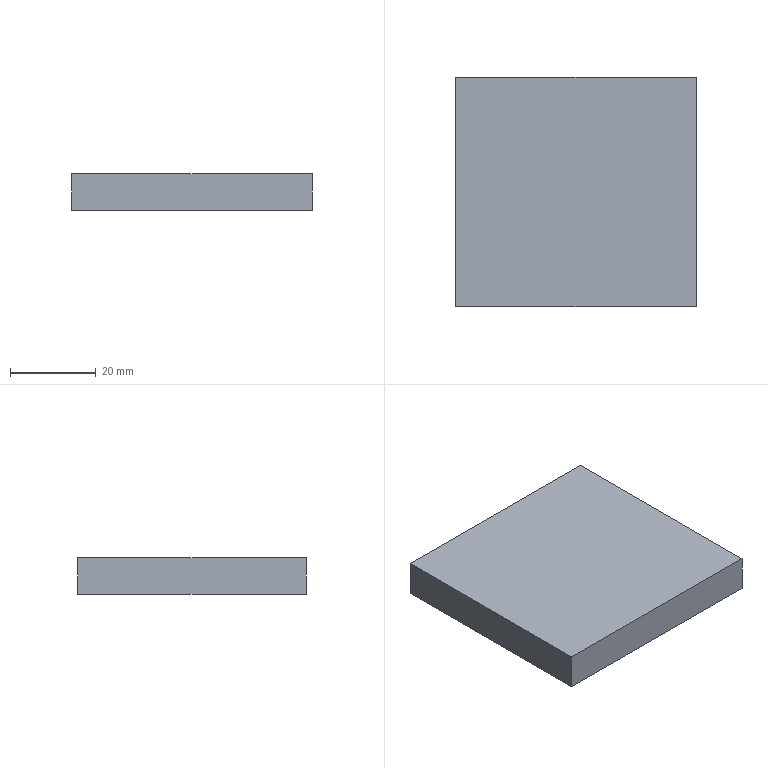NC program | NX | posted with a generic post | part box 56 x 53.3 x 8.5 mm
Lines 1846 to 3579 of 5023, first 1622 of 1730 lines:
(CAVITY_MILL_COPY , TOOL : D4)
N3678 T11 M6
N3680 G54
N3682 G17 G0 G90 X8.296 Y14.357 S9500 M3
N3684 G43 Z30. H11
N3686 Z-0.75
N3688 G94 G1 Z-1.75 F800.
N3690 X8.533 Y14.434
N3692 G3 X9.2 Y15.179 R1.
N3694 G2 X9.473 Y16.065 R5.05 F1200.
N3696 G3 X8.615 Y16.541 R18.65
N3698 X7.615 Y16.498 R1.
N3700 G1 X7.293 Y16.292
N3702 Z-0.75
N3704 X8.296 Y14.357 Z-1. F6000.
N3706 Z-2. F800.
N3708 X8.533 Y14.434
N3710 G3 X9.2 Y15.179 R1.
N3712 G2 X9.473 Y16.065 R5.05 F1200.
N3714 G3 X8.615 Y16.541 R18.65
N3716 X7.615 Y16.498 R1.
N3718 G1 X7.293 Y16.292
N3720 Z-1.
N3722 X8.296 Y14.357 Z-1.25 F6000.
N3724 Z-2.25 F800.
N3726 X8.533 Y14.434
N3728 G3 X9.2 Y15.179 R1.
N3730 G2 X9.473 Y16.065 R5.05 F1200.
N3732 G3 X8.615 Y16.541 R18.65
N3734 X7.615 Y16.498 R1.
N3736 G1 X7.293 Y16.292
N3738 Z-1.25
N3740 X8.296 Y14.357 Z-1.5 F6000.
N3742 Z-2.5 F800.
N3744 X8.533 Y14.434
N3746 G3 X9.2 Y15.179 R1.
N3748 G2 X9.473 Y16.065 R5.05 F1200.
N3750 G3 X8.615 Y16.541 R18.65
N3752 X7.615 Y16.498 R1.
N3754 G1 X7.293 Y16.292
N3756 Z-1.5
N3758 G0 Z30.
N3760 X15.388 Y16.801
N3762 Z-0.75
N3764 G1 Z-1.75 F800.
N3766 X15.171 Y16.699
N3768 G3 X14.599 Y15.878 R1.
N3770 G2 X14.098 Y14.165 R4.5 F1200.
N3772 G1 X14.072 Y14.116
N3774 X14.116 Y14.072
N3776 X14.165 Y14.098
N3778 G2 X15.878 Y14.599 R4.5
N3780 G3 X16.699 Y15.171 R1.
N3782 G1 X16.801 Y15.388
N3784 Z-0.75
N3786 X15.388 Y16.801 Z-1. F6000.
N3788 Z-2. F800.
N3790 X15.171 Y16.699
N3792 G3 X14.599 Y15.878 R1.
N3794 G2 X14.098 Y14.165 R4.5 F1200.
N3796 G1 X14.072 Y14.116
N3798 X14.116 Y14.072
N3800 X14.165 Y14.098
N3802 G2 X15.878 Y14.599 R4.5
N3804 G3 X16.699 Y15.171 R1.
N3806 G1 X16.801 Y15.388
N3808 Z-1.
N3810 X15.388 Y16.801 Z-1.25 F6000.
N3812 Z-2.25 F800.
N3814 X15.171 Y16.699
N3816 G3 X14.599 Y15.878 R1.
N3818 G2 X14.098 Y14.165 R4.5 F1200.
N3820 G1 X14.072 Y14.116
N3822 X14.116 Y14.072
N3824 X14.165 Y14.098
N3826 G2 X15.878 Y14.599 R4.5
N3828 G3 X16.699 Y15.171 R1.
N3830 G1 X16.801 Y15.388
N3832 Z-1.25
N3834 X15.388 Y16.801 Z-1.5 F6000.
N3836 Z-2.5 F800.
N3838 X15.171 Y16.699
N3840 G3 X14.599 Y15.878 R1.
N3842 G2 X14.098 Y14.165 R4.5 F1200.
N3844 G1 X14.072 Y14.116
N3846 X14.116 Y14.072
N3848 X14.165 Y14.098
N3850 G2 X15.878 Y14.599 R4.5
N3852 G3 X16.699 Y15.171 R1.
N3854 G1 X16.801 Y15.388
N3856 Z-1.5
N3858 X15.388 Y16.801 Z-1.8 F6000.
N3860 Z-2.8 F800.
N3862 X15.171 Y16.699
N3864 G3 X14.599 Y15.878 R1.
N3866 G2 X14.098 Y14.165 R4.5 F1200.
N3868 G1 X14.072 Y14.116
N3870 X14.116 Y14.072
N3872 X14.165 Y14.098
N3874 G2 X15.878 Y14.599 R4.5
N3876 G3 X16.699 Y15.171 R1.
N3878 G1 X16.801 Y15.388
N3880 Z-1.8
N3882 X15.388 Y16.801 Z-2.1 F6000.
N3884 Z-3.1 F800.
N3886 X15.171 Y16.699
N3888 G3 X14.599 Y15.878 R1.
N3890 G2 X14.098 Y14.165 R4.5 F1200.
N3892 G1 X14.072 Y14.116
N3894 X14.116 Y14.072
N3896 X14.165 Y14.098
N3898 G2 X15.878 Y14.599 R4.5
N3900 G3 X16.699 Y15.171 R1.
N3902 G1 X16.801 Y15.388
N3904 Z-2.1
N3906 X15.388 Y16.801 Z-2.3 F6000.
N3908 Z-3.3 F800.
N3910 X15.171 Y16.699
N3912 G3 X14.599 Y15.878 R1.
N3914 G2 X14.098 Y14.165 R4.5 F1200.
N3916 G1 X14.072 Y14.116
N3918 X14.116 Y14.072
N3920 X14.165 Y14.098
N3922 G2 X15.878 Y14.599 R4.5
N3924 G3 X16.699 Y15.171 R1.
N3926 G1 X16.801 Y15.388
N3928 Z-2.3
N3930 X15.388 Y16.801 Z-2.5 F6000.
N3932 Z-3.5 F800.
N3934 X15.171 Y16.699
N3936 G3 X14.599 Y15.878 R1.
N3938 G2 X14.098 Y14.165 R4.5 F1200.
N3940 G1 X14.072 Y14.116
N3942 X14.116 Y14.072
N3944 X14.165 Y14.098
N3946 G2 X15.878 Y14.599 R4.5
N3948 G3 X16.699 Y15.171 R1.
N3950 G1 X16.801 Y15.388
N3952 Z-2.5
N3954 G0 Z30.
N3956 X16.292 Y7.293
N3958 Z-0.75
N3960 G1 Z-1.75 F800.
N3962 X16.498 Y7.615
N3964 G3 X16.541 Y8.615 R1.
N3966 X16.065 Y9.473 R18.65 F1200.
N3968 G2 X15.179 Y9.2 R5.05
N3970 G3 X14.434 Y8.533 R1.
N3972 G1 X14.357 Y8.296
N3974 Z-0.75
N3976 X16.292 Y7.293 Z-1. F6000.
N3978 Z-2. F800.
N3980 X16.498 Y7.615
N3982 G3 X16.541 Y8.615 R1.
N3984 X16.065 Y9.473 R18.65 F1200.
N3986 G2 X15.179 Y9.2 R5.05
N3988 G3 X14.434 Y8.533 R1.
N3990 G1 X14.357 Y8.296
N3992 Z-1.
N3994 X16.292 Y7.293 Z-1.25 F6000.
N3996 Z-2.25 F800.
N3998 X16.498 Y7.615
N4000 G3 X16.541 Y8.615 R1.
N4002 X16.065 Y9.473 R18.65 F1200.
N4004 G2 X15.179 Y9.2 R5.05
N4006 G3 X14.434 Y8.533 R1.
N4008 G1 X14.357 Y8.296
N4010 Z-1.25
N4012 X16.292 Y7.293 Z-1.5 F6000.
N4014 Z-2.5 F800.
N4016 X16.498 Y7.615
N4018 G3 X16.541 Y8.615 R1.
N4020 X16.065 Y9.473 R18.65 F1200.
N4022 G2 X15.179 Y9.2 R5.05
N4024 G3 X14.434 Y8.533 R1.
N4026 G1 X14.357 Y8.296
N4028 Z-1.5
N4030 G0 Z30.
N4032 X21.661 Y11.34
N4034 Z-0.75
N4036 G1 Z-1.75 F800.
N4038 X21.478 Y11.076
N4040 G3 X21.394 Y10.08 R1.
N4042 G2 X21.665 Y9.484 R23.65 F1200.
N4044 X22.28 Y9.334 R2.5
N4046 G3 X23.267 Y9.49 R1.
N4048 G1 X23.409 Y9.605
N4050 Z-0.75
N4052 X21.661 Y11.34 Z-1. F6000.
N4054 Z-2. F800.
N4056 X21.478 Y11.076
N4058 G3 X21.394 Y10.08 R1.
N4060 G2 X21.665 Y9.484 R23.65 F1200.
N4062 X22.28 Y9.334 R2.5
N4064 G3 X23.267 Y9.49 R1.
N4066 G1 X23.409 Y9.605
N4068 Z-1.
N4070 X21.661 Y11.34 Z-1.25 F6000.
N4072 Z-2.25 F800.
N4074 X21.478 Y11.076
N4076 G3 X21.394 Y10.08 R1.
N4078 G2 X21.665 Y9.484 R23.65 F1200.
N4080 X22.28 Y9.334 R2.5
N4082 G3 X23.267 Y9.49 R1.
N4084 G1 X23.409 Y9.605
N4086 Z-1.25
N4088 X21.661 Y11.34 Z-1.5 F6000.
N4090 Z-2.5 F800.
N4092 X21.478 Y11.076
N4094 G3 X21.394 Y10.08 R1.
N4096 G2 X21.665 Y9.484 R23.65 F1200.
N4098 X22.28 Y9.334 R2.5
N4100 G3 X23.267 Y9.49 R1.
N4102 G1 X23.409 Y9.605
N4104 Z-1.5
N4106 X21.661 Y11.34 Z-1.8 F6000.
N4108 Z-2.8 F800.
N4110 X21.478 Y11.076
N4112 G3 X21.394 Y10.08 R1.
N4114 G2 X21.665 Y9.484 R23.65 F1200.
N4116 X22.28 Y9.334 R2.5
N4118 G3 X23.267 Y9.49 R1.
N4120 G1 X23.409 Y9.605
N4122 Z-1.8
N4124 X21.661 Y11.34 Z-2.1 F6000.
N4126 Z-3.1 F800.
N4128 X21.478 Y11.076
N4130 G3 X21.394 Y10.08 R1.
N4132 G2 X21.665 Y9.484 R23.65 F1200.
N4134 X22.28 Y9.334 R2.5
N4136 G3 X23.267 Y9.49 R1.
N4138 G1 X23.409 Y9.605
N4140 Z-2.1
N4142 X21.661 Y11.34 Z-2.3 F6000.
N4144 Z-3.3 F800.
N4146 X21.478 Y11.076
N4148 G3 X21.394 Y10.08 R1.
N4150 G2 X21.665 Y9.484 R23.65 F1200.
N4152 X22.28 Y9.334 R2.5
N4154 G3 X23.267 Y9.49 R1.
N4156 G1 X23.409 Y9.605
N4158 Z-2.3
N4160 X21.661 Y11.34 Z-2.5 F6000.
N4162 Z-3.5 F800.
N4164 X21.478 Y11.076
N4166 G3 X21.394 Y10.08 R1.
N4168 G2 X21.665 Y9.484 R23.65 F1200.
N4170 X22.28 Y9.334 R2.5
N4172 G3 X23.267 Y9.49 R1.
N4174 G1 X23.409 Y9.605
N4176 Z-2.5
N4178 G0 Z30.
N4180 X18.956 Y3.051
N4182 Z-0.75
N4184 G1 Z-1.75 F800.
N4186 X19.237 Y3.306
N4188 G3 X19.541 Y4.259 R1.
N4190 X19.4 Y4.863 R20. F1200.
N4192 G2 X18.864 Y5.142 R4.
N4194 G3 X17.865 Y5.176 R1.
N4196 G1 X17.662 Y5.068
N4198 Z-0.75
N4200 X18.956 Y3.051 Z-1. F6000.
N4202 Z-2. F800.
N4204 X19.237 Y3.306
N4206 G3 X19.541 Y4.259 R1.
N4208 X19.4 Y4.863 R20. F1200.
N4210 G2 X18.864 Y5.142 R4.
N4212 G3 X17.865 Y5.176 R1.
N4214 G1 X17.662 Y5.068
N4216 Z-1.
N4218 X18.956 Y3.05 Z-1.25 F6000.
N4220 Z-2.25 F800.
N4222 X19.237 Y3.306
N4224 G3 X19.541 Y4.259 R1.
N4226 X19.4 Y4.863 R20. F1200.
N4228 G2 X18.864 Y5.143 R4.
N4230 G3 X17.865 Y5.176 R1.
N4232 G1 X17.662 Y5.068
N4234 Z-1.25
N4236 X18.956 Y3.05 Z-1.5 F6000.
N4238 Z-2.5 F800.
N4240 X19.237 Y3.306
N4242 G3 X19.541 Y4.259 R1.
N4244 X19.4 Y4.863 R20. F1200.
N4246 G2 X18.864 Y5.143 R4.
N4248 G3 X17.865 Y5.176 R1.
N4250 G1 X17.662 Y5.068
N4252 Z-1.5
N4254 X17. Y1.805 F6000.
N4256 Y0.5 Z-1.568 F800.
N4258 X19. Z-1.673
N4260 Y3.5 Z-1.83
N4262 X17. Z-1.935
N4264 Y0.5 Z-2.092
N4266 X19. Z-2.197
N4268 Y3.5 Z-2.355
N4270 X17. Z-2.459
N4272 Y0.5 Z-2.617
N4274 X19. Z-2.721
N4276 Y2. Z-2.8
N4278 Y3.5 F1200.
N4280 X17.
N4282 Y0.5
N4284 X19.
N4286 Y2.
N4288 G3 X18.5 Y2.866 R1.
N4290 G1 Z-1.8
N4292 X17. Y1.805 F6000.
N4294 Y0.5 Z-1.868 F800.
N4296 X19. Z-1.973
N4298 Y3.5 Z-2.13
N4300 X17. Z-2.235
N4302 Y0.5 Z-2.392
N4304 X19. Z-2.497
N4306 Y3.5 Z-2.655
N4308 X17. Z-2.759
N4310 Y0.5 Z-2.917
N4312 X19. Z-3.021
N4314 Y2. Z-3.1
N4316 Y3.5 F1200.
N4318 X17.
N4320 Y0.5
N4322 X19.
N4324 Y2.
N4326 G3 X18.5 Y2.866 R1.
N4328 G1 Z-2.1
N4330 G0 Z30.
N4332 X17.122 Y-4.78
N4334 Z-0.75
N4336 G1 Z-1.75 F800.
N4338 X17.865 Y-5.176
N4340 G3 X18.864 Y-5.142 R1.
N4342 G2 X19.4 Y-4.863 R4. F1200.
N4344 G3 X19.541 Y-4.259 R20.
N4346 X19.237 Y-3.307 R1.
N4348 G1 X18.956 Y-3.051
N4350 Z-0.75
N4352 X17.122 Y-4.78 Z-1. F6000.
N4354 Z-2. F800.
N4356 X17.865 Y-5.176
N4358 G3 X18.864 Y-5.142 R1.
N4360 G2 X19.4 Y-4.863 R4. F1200.
N4362 G3 X19.541 Y-4.259 R20.
N4364 X19.237 Y-3.307 R1.
N4366 G1 X18.956 Y-3.051
N4368 Z-1.
N4370 X17.122 Y-4.78 Z-1.25 F6000.
N4372 Z-2.25 F800.
N4374 X17.865 Y-5.176
N4376 G3 X18.864 Y-5.142 R1.
N4378 G2 X19.4 Y-4.863 R4. F1200.
N4380 G3 X19.541 Y-4.259 R20.
N4382 X19.237 Y-3.307 R1.
N4384 G1 X18.956 Y-3.051
N4386 Z-1.25
N4388 X17.122 Y-4.78 Z-1.5 F6000.
N4390 Z-2.5 F800.
N4392 X17.865 Y-5.176
N4394 G3 X18.864 Y-5.142 R1.
N4396 G2 X19.4 Y-4.863 R4. F1200.
N4398 G3 X19.541 Y-4.259 R20.
N4400 X19.237 Y-3.307 R1.
N4402 G1 X18.956 Y-3.051
N4404 Z-1.5
N4406 G0 Z30.
N4408 X16.237 Y-4.956
N4410 Z-0.75
N4412 G1 Z-1.75 F800.
N4414 X16.302 Y-5.181
N4416 G3 X17.023 Y-5.875 R1.
N4418 G2 X17.778 Y-6.14 R4.25 F1200.
N4420 X18.318 Y-5.552 R4.
N4422 G3 X18.631 Y-4.602 R1.
N4424 G1 X18.478 Y-3.86
N4426 Z-0.75
N4428 X16.237 Y-4.956 Z-1. F6000.
N4430 Z-2. F800.
N4432 X16.302 Y-5.181
N4434 G3 X17.023 Y-5.875 R1.
N4436 G2 X17.778 Y-6.14 R4.25 F1200.
N4438 X18.318 Y-5.552 R4.
N4440 G3 X18.631 Y-4.602 R1.
N4442 G1 X18.478 Y-3.86
N4444 Z-1.
N4446 X16.237 Y-4.956 Z-1.25 F6000.
N4448 Z-2.25 F800.
N4450 X16.302 Y-5.181
N4452 G3 X17.023 Y-5.875 R1.
N4454 G2 X17.778 Y-6.14 R4.25 F1200.
N4456 X18.318 Y-5.552 R4.
N4458 G3 X18.631 Y-4.602 R1.
N4460 G1 X18.478 Y-3.86
N4462 Z-1.25
N4464 X16.237 Y-4.956 Z-1.5 F6000.
N4466 Z-2.5 F800.
N4468 X16.302 Y-5.181
N4470 G3 X17.023 Y-5.875 R1.
N4472 G2 X17.778 Y-6.14 R4.25 F1200.
N4474 X18.318 Y-5.552 R4.
N4476 G3 X18.631 Y-4.602 R1.
N4478 G1 X18.478 Y-3.86
N4480 Z-1.5
N4482 G0 Z30.
N4484 X23.409 Y-9.605
N4486 Z-0.75
N4488 G1 Z-1.75 F800.
N4490 X23.267 Y-9.49
N4492 G3 X22.279 Y-9.334 R1.
N4494 G2 X21.665 Y-9.484 R2.5 F1200.
N4496 X21.394 Y-10.08 R23.65
N4498 G3 X21.478 Y-11.076 R1.
N4500 G1 X21.661 Y-11.34
N4502 Z-0.75
N4504 X23.409 Y-9.605 Z-1. F6000.
N4506 Z-2. F800.
N4508 X23.267 Y-9.49
N4510 G3 X22.279 Y-9.334 R1.
N4512 G2 X21.665 Y-9.484 R2.5 F1200.
N4514 X21.394 Y-10.08 R23.65
N4516 G3 X21.478 Y-11.076 R1.
N4518 G1 X21.661 Y-11.34
N4520 Z-1.
N4522 X23.409 Y-9.605 Z-1.25 F6000.
N4524 Z-2.25 F800.
N4526 X23.267 Y-9.49
N4528 G3 X22.279 Y-9.334 R1.
N4530 G2 X21.665 Y-9.484 R2.5 F1200.
N4532 X21.394 Y-10.08 R23.65
N4534 G3 X21.478 Y-11.076 R1.
N4536 G1 X21.661 Y-11.34
N4538 Z-1.25
N4540 X23.409 Y-9.605 Z-1.5 F6000.
N4542 Z-2.5 F800.
N4544 X23.267 Y-9.49
N4546 G3 X22.279 Y-9.334 R1.
N4548 G2 X21.665 Y-9.484 R2.5 F1200.
N4550 X21.394 Y-10.08 R23.65
N4552 G3 X21.478 Y-11.076 R1.
N4554 G1 X21.661 Y-11.34
N4556 Z-1.5
N4558 X23.409 Y-9.605 Z-1.8 F6000.
N4560 Z-2.8 F800.
N4562 X23.267 Y-9.49
N4564 G3 X22.279 Y-9.334 R1.
N4566 G2 X21.665 Y-9.484 R2.5 F1200.
N4568 X21.394 Y-10.08 R23.65
N4570 G3 X21.478 Y-11.076 R1.
N4572 G1 X21.661 Y-11.34
N4574 Z-1.8
N4576 X23.409 Y-9.605 Z-2.1 F6000.
N4578 Z-3.1 F800.
N4580 X23.267 Y-9.49
N4582 G3 X22.279 Y-9.334 R1.
N4584 G2 X21.665 Y-9.484 R2.5 F1200.
N4586 X21.394 Y-10.08 R23.65
N4588 G3 X21.478 Y-11.076 R1.
N4590 G1 X21.661 Y-11.34
N4592 Z-2.1
N4594 X23.409 Y-9.605 Z-2.3 F6000.
N4596 Z-3.3 F800.
N4598 X23.267 Y-9.49
N4600 G3 X22.279 Y-9.334 R1.
N4602 G2 X21.665 Y-9.484 R2.5 F1200.
N4604 X21.394 Y-10.08 R23.65
N4606 G3 X21.478 Y-11.076 R1.
N4608 G1 X21.661 Y-11.34
N4610 Z-2.3
N4612 X23.409 Y-9.605 Z-2.5 F6000.
N4614 Z-3.5 F800.
N4616 X23.267 Y-9.49
N4618 G3 X22.279 Y-9.334 R1.
N4620 G2 X21.665 Y-9.484 R2.5 F1200.
N4622 X21.394 Y-10.08 R23.65
N4624 G3 X21.478 Y-11.076 R1.
N4626 G1 X21.661 Y-11.34
N4628 Z-2.5
N4630 G0 Z30.
N4632 X16.801 Y-15.388
N4634 Z-0.75
N4636 G1 Z-1.75 F800.
N4638 X16.699 Y-15.171
N4640 G3 X15.878 Y-14.599 R1.
N4642 G2 X14.165 Y-14.098 R4.5 F1200.
N4644 G1 X14.116 Y-14.072
N4646 X14.072 Y-14.116
N4648 X14.098 Y-14.165
N4650 G2 X14.599 Y-15.878 R4.5
N4652 G3 X15.171 Y-16.699 R1.
N4654 G1 X15.388 Y-16.801
N4656 Z-0.75
N4658 X16.801 Y-15.388 Z-1. F6000.
N4660 Z-2. F800.
N4662 X16.699 Y-15.171
N4664 G3 X15.878 Y-14.599 R1.
N4666 G2 X14.165 Y-14.098 R4.5 F1200.
N4668 G1 X14.116 Y-14.072
N4670 X14.072 Y-14.116
N4672 X14.098 Y-14.165
N4674 G2 X14.599 Y-15.878 R4.5
N4676 G3 X15.171 Y-16.699 R1.
N4678 G1 X15.388 Y-16.801
N4680 Z-1.
N4682 X16.801 Y-15.388 Z-1.25 F6000.
N4684 Z-2.25 F800.
N4686 X16.699 Y-15.171
N4688 G3 X15.878 Y-14.599 R1.
N4690 G2 X14.165 Y-14.098 R4.5 F1200.
N4692 G1 X14.116 Y-14.072
N4694 X14.072 Y-14.116
N4696 X14.098 Y-14.165
N4698 G2 X14.599 Y-15.878 R4.5
N4700 G3 X15.171 Y-16.699 R1.
N4702 G1 X15.388 Y-16.801
N4704 Z-1.25
N4706 X16.801 Y-15.388 Z-1.5 F6000.
N4708 Z-2.5 F800.
N4710 X16.699 Y-15.171
N4712 G3 X15.878 Y-14.599 R1.
N4714 G2 X14.165 Y-14.098 R4.5 F1200.
N4716 G1 X14.116 Y-14.072
N4718 X14.072 Y-14.116
N4720 X14.098 Y-14.165
N4722 G2 X14.599 Y-15.878 R4.5
N4724 G3 X15.171 Y-16.699 R1.
N4726 G1 X15.388 Y-16.801
N4728 Z-1.5
N4730 X16.801 Y-15.388 Z-1.8 F6000.
N4732 Z-2.8 F800.
N4734 X16.699 Y-15.171
N4736 G3 X15.878 Y-14.599 R1.
N4738 G2 X14.165 Y-14.098 R4.5 F1200.
N4740 G1 X14.116 Y-14.072
N4742 X14.072 Y-14.116
N4744 X14.098 Y-14.165
N4746 G2 X14.599 Y-15.878 R4.5
N4748 G3 X15.171 Y-16.699 R1.
N4750 G1 X15.388 Y-16.801
N4752 Z-1.8
N4754 X16.801 Y-15.388 Z-2.1 F6000.
N4756 Z-3.1 F800.
N4758 X16.699 Y-15.171
N4760 G3 X15.878 Y-14.599 R1.
N4762 G2 X14.165 Y-14.098 R4.5 F1200.
N4764 G1 X14.116 Y-14.072
N4766 X14.072 Y-14.116
N4768 X14.098 Y-14.165
N4770 G2 X14.599 Y-15.878 R4.5
N4772 G3 X15.171 Y-16.699 R1.
N4774 G1 X15.388 Y-16.801
N4776 Z-2.1
N4778 X16.801 Y-15.388 Z-2.3 F6000.
N4780 Z-3.3 F800.
N4782 X16.699 Y-15.171
N4784 G3 X15.878 Y-14.599 R1.
N4786 G2 X14.165 Y-14.098 R4.5 F1200.
N4788 G1 X14.116 Y-14.072
N4790 X14.072 Y-14.116
N4792 X14.098 Y-14.165
N4794 G2 X14.599 Y-15.878 R4.5
N4796 G3 X15.171 Y-16.699 R1.
N4798 G1 X15.388 Y-16.801
N4800 Z-2.3
N4802 X16.801 Y-15.388 Z-2.5 F6000.
N4804 Z-3.5 F800.
N4806 X16.699 Y-15.171
N4808 G3 X15.878 Y-14.599 R1.
N4810 G2 X14.165 Y-14.098 R4.5 F1200.
N4812 G1 X14.116 Y-14.072
N4814 X14.072 Y-14.116
N4816 X14.098 Y-14.165
N4818 G2 X14.599 Y-15.878 R4.5
N4820 G3 X15.171 Y-16.699 R1.
N4822 G1 X15.388 Y-16.801
N4824 Z-2.5
N4826 G0 Z30.
N4828 X11.3 Y-6.108
N4830 Z-0.75
N4832 G1 Z-1.75 F800.
N4834 X11. Y-6.281
N4836 G3 X10.5 Y-7.147 R1.
N4838 G1 Y-10. F1200.
N4840 X11.253
N4842 G2 X11.761 Y-9.689 R5.05
N4844 X12.455 Y-7.655 R4.25
N4846 G3 X12.516 Y-6.657 R1.
N4848 G1 X12.411 Y-6.447
N4850 Z-0.75
N4852 X11.3 Y-6.108 Z-1. F6000.
N4854 Z-2. F800.
N4856 X11. Y-6.281
N4858 G3 X10.5 Y-7.147 R1.
N4860 G1 Y-10. F1200.
N4862 X11.254
N4864 G2 X11.761 Y-9.689 R5.05
N4866 X12.455 Y-7.655 R4.25
N4868 G3 X12.516 Y-6.657 R1.
N4870 G1 X12.411 Y-6.447
N4872 Z-1.
N4874 X11.3 Y-6.108 Z-1.25 F6000.
N4876 Z-2.25 F800.
N4878 X11. Y-6.281
N4880 G3 X10.5 Y-7.147 R1.
N4882 G1 Y-10. F1200.
N4884 X11.254
N4886 G2 X11.761 Y-9.689 R5.05
N4888 X12.455 Y-7.655 R4.25
N4890 G3 X12.516 Y-6.657 R1.
N4892 G1 X12.411 Y-6.447
N4894 Z-1.25
N4896 X11.3 Y-6.108 Z-1.5 F6000.
N4898 Z-2.5 F800.
N4900 X11. Y-6.281
N4902 G3 X10.5 Y-7.147 R1.
N4904 G1 Y-10. F1200.
N4906 X11.254
N4908 G2 X11.761 Y-9.689 R5.05
N4910 X12.455 Y-7.655 R4.25
N4912 G3 X12.516 Y-6.657 R1.
N4914 G1 X12.411 Y-6.447
N4916 Z-1.5
N4918 G0 Z30.
N4920 X-3.336 Y-18.35
N4922 Z1.
N4924 G1 X-1.295 Y-18.635 Z0.892 F800.
N4926 X1.295 Z0.756
N4928 X3.859 Y-18.277 Z0.621
N4930 X4.881 Y-18. Z0.565
N4932 X-4.881 Z0.054
N4934 X-3.859 Y-18.277 Z-0.002
N4936 X-1.295 Y-18.635 Z-0.138
N4938 X1.295 Z-0.273
N4940 X3.859 Y-18.277 Z-0.409
N4942 X4.881 Y-18. Z-0.465
N4944 X-4.881 Z-0.976
N4946 X-3.859 Y-18.277 Z-1.032
N4948 X-1.295 Y-18.635 Z-1.167
N4950 X1.295 Z-1.303
N4952 X3.859 Y-18.277 Z-1.439
N4954 X4.881 Y-18. Z-1.494
N4956 X0. Z-1.75
N4958 X-4.881 F1200.
N4960 G3 X4.881 Y-18. R18.65
N4962 G1 X0.
N4964 G3 X-0.866 Y-18.5 R1.
N4966 G1 Z-0.75
N4968 X4.205 Y-18. F6000.
N4970 X-4.881 Z-1.226 F800.
N4972 X-3.859 Y-18.277 Z-1.282
N4974 X-1.295 Y-18.635 Z-1.417
N4976 X1.295 Z-1.553
N4978 X3.859 Y-18.277 Z-1.689
N4980 X4.881 Y-18. Z-1.744
N4982 X0. Z-2.
N4984 X-4.881 F1200.
N4986 G3 X4.881 Y-18. R18.65
N4988 G1 X0.
N4990 G3 X-0.866 Y-18.5 R1.
N4992 G1 Z-1.
N4994 X4.205 Y-18. F6000.
N4996 X-4.881 Z-1.476 F800.
N4998 X-3.859 Y-18.277 Z-1.532
N5000 X-1.295 Y-18.635 Z-1.667
N5002 X1.295 Z-1.803
N5004 X3.859 Y-18.277 Z-1.939
N5006 X4.881 Y-18. Z-1.994
N5008 X0. Z-2.25
N5010 X-4.881 F1200.
N5012 G3 X4.881 Y-18. R18.65
N5014 G1 X0.
N5016 G3 X-0.866 Y-18.5 R1.
N5018 G1 Z-1.25
N5020 X4.205 Y-18. F6000.
N5022 X-4.881 Z-1.726 F800.
N5024 X-3.859 Y-18.277 Z-1.782
N5026 X-1.295 Y-18.635 Z-1.917
N5028 X1.295 Z-2.053
N5030 X3.859 Y-18.277 Z-2.189
N5032 X4.881 Y-18. Z-2.244
N5034 X0. Z-2.5
N5036 X-4.881 F1200.
N5038 G3 X4.881 Y-18. R18.65
N5040 G1 X0.
N5042 G3 X-0.866 Y-18.5 R1.
N5044 G1 Z-1.5
N5046 G0 Z30.
N5048 X-12.715 Y-8.469
N5050 Z-0.75
N5052 G1 Z-1.75 F800.
N5054 X-12.689 Y-8.716
N5056 G3 X-12.099 Y-9.524 R1.
N5058 G2 X-11.253 Y-10. R5.05 F1200.
N5060 G1 X-10.5
N5062 Y-8.551
N5064 G3 X-11. Y-7.685 R1.
N5066 G1 X-11.3 Y-7.512
N5068 Z-0.75
N5070 X-12.715 Y-8.469 Z-1. F6000.
N5072 Z-2. F800.
N5074 X-12.689 Y-8.716
N5076 G3 X-12.099 Y-9.524 R1.
N5078 G2 X-11.253 Y-10. R5.05 F1200.
N5080 G1 X-10.5
N5082 Y-8.551
N5084 G3 X-11. Y-7.685 R1.
N5086 G1 X-11.3 Y-7.512
N5088 Z-1.
N5090 X-12.715 Y-8.469 Z-1.25 F6000.
N5092 Z-2.25 F800.
N5094 X-12.689 Y-8.716
N5096 G3 X-12.099 Y-9.524 R1.
N5098 G2 X-11.253 Y-10. R5.05 F1200.
N5100 G1 X-10.5
N5102 Y-8.551
N5104 G3 X-11. Y-7.685 R1.
N5106 G1 X-11.3 Y-7.512
N5108 Z-1.25
N5110 X-12.715 Y-8.469 Z-1.5 F6000.
N5112 Z-2.5 F800.
N5114 X-12.689 Y-8.716
N5116 G3 X-12.099 Y-9.524 R1.
N5118 G2 X-11.253 Y-10. R5.05 F1200.
N5120 G1 X-10.5
N5122 Y-8.551
N5124 G3 X-11. Y-7.685 R1.
N5126 G1 X-11.3 Y-7.512
N5128 Z-1.5
N5130 G0 Z30.
N5132 X-15.388 Y-16.801
N5134 Z-0.75
N5136 G1 Z-1.75 F800.
N5138 X-15.171 Y-16.699
N5140 G3 X-14.599 Y-15.878 R1.
N5142 G2 X-14.098 Y-14.165 R4.5 F1200.
N5144 G1 X-14.072 Y-14.117
N5146 X-14.113 Y-14.073
N5148 X-14.163 Y-14.097
N5150 X-14.244 Y-14.138
N5152 G2 X-15.878 Y-14.599 R4.5
N5154 G3 X-16.699 Y-15.171 R1.
N5156 G1 X-16.801 Y-15.388
N5158 Z-0.75
N5160 X-15.388 Y-16.801 Z-1. F6000.
N5162 Z-2. F800.
N5164 X-15.171 Y-16.699
N5166 G3 X-14.599 Y-15.878 R1.
N5168 G2 X-14.098 Y-14.165 R4.5 F1200.
N5170 G1 X-14.072 Y-14.117
N5172 X-14.114 Y-14.073
N5174 X-14.163 Y-14.097
N5176 X-14.236 Y-14.134
N5178 G2 X-15.878 Y-14.599 R4.5
N5180 G3 X-16.699 Y-15.171 R1.
N5182 G1 X-16.801 Y-15.388
N5184 Z-1.
N5186 X-15.388 Y-16.801 Z-1.25 F6000.
N5188 Z-2.25 F800.
N5190 X-15.171 Y-16.699
N5192 G3 X-14.599 Y-15.878 R1.
N5194 G2 X-14.098 Y-14.165 R4.5 F1200.
N5196 G1 X-14.072 Y-14.116
N5198 X-14.114 Y-14.073
N5200 X-14.164 Y-14.097
N5202 X-14.228 Y-14.13
N5204 G2 X-15.878 Y-14.599 R4.5
N5206 G3 X-16.699 Y-15.171 R1.
N5208 G1 X-16.801 Y-15.388
N5210 Z-1.25
N5212 X-15.388 Y-16.801 Z-1.5 F6000.
N5214 Z-2.5 F800.
N5216 X-15.171 Y-16.699
N5218 G3 X-14.599 Y-15.878 R1.
N5220 G2 X-14.098 Y-14.165 R4.5 F1200.
N5222 G1 X-14.072 Y-14.116
N5224 X-14.114 Y-14.072
N5226 X-14.164 Y-14.097
N5228 X-14.218 Y-14.125
N5230 G2 X-15.878 Y-14.599 R4.5
N5232 G3 X-16.699 Y-15.171 R1.
N5234 G1 X-16.801 Y-15.388
N5236 Z-1.5
N5238 X-15.388 Y-16.801 Z-1.8 F6000.
N5240 Z-2.8 F800.
N5242 X-15.171 Y-16.699
N5244 G3 X-14.599 Y-15.878 R1.
N5246 G2 X-14.098 Y-14.165 R4.5 F1200.
N5248 G1 X-14.072 Y-14.116
N5250 X-14.115 Y-14.072
N5252 X-14.165 Y-14.098
N5254 X-14.202 Y-14.117
N5256 G2 X-15.878 Y-14.599 R4.5
N5258 G3 X-16.699 Y-15.171 R1.
N5260 G1 X-16.801 Y-15.388
N5262 Z-1.8
N5264 X-15.388 Y-16.801 Z-2.1 F6000.
N5266 Z-3.1 F800.
N5268 X-15.171 Y-16.699
N5270 G3 X-14.599 Y-15.878 R1.
N5272 G2 X-14.098 Y-14.165 R4.5 F1200.
N5274 G1 X-14.165 Y-14.098
N5276 G2 X-15.878 Y-14.599 R4.5
N5278 G3 X-16.699 Y-15.171 R1.
N5280 G1 X-16.801 Y-15.388
N5282 Z-2.1
N5284 X-15.388 Y-16.801 Z-2.3 F6000.
N5286 Z-3.3 F800.
N5288 X-15.171 Y-16.699
N5290 G3 X-14.599 Y-15.878 R1.
N5292 G2 X-14.098 Y-14.165 R4.5 F1200.
N5294 G1 X-14.166 Y-14.098
N5296 G2 X-15.878 Y-14.599 R4.5
N5298 G3 X-16.699 Y-15.171 R1.
N5300 G1 X-16.801 Y-15.388
N5302 Z-2.3
N5304 X-15.388 Y-16.801 Z-2.5 F6000.
N5306 Z-3.5 F800.
N5308 X-15.171 Y-16.699
N5310 G3 X-14.599 Y-15.878 R1.
N5312 G2 X-14.098 Y-14.165 R4.5 F1200.
N5314 G1 X-14.166 Y-14.098
N5316 G2 X-15.878 Y-14.599 R4.5
N5318 G3 X-16.699 Y-15.171 R1.
N5320 G1 X-16.801 Y-15.388
N5322 Z-2.5
N5324 G0 Z30.
N5326 X-16.292 Y-7.293
N5328 Z-0.75
N5330 G1 Z-1.75 F800.
N5332 X-16.498 Y-7.615
N5334 G3 X-16.541 Y-8.615 R1.
N5336 X-16.065 Y-9.473 R18.65 F1200.
N5338 G2 X-15.179 Y-9.2 R5.05
N5340 G3 X-14.434 Y-8.533 R1.
N5342 G1 X-14.357 Y-8.296
N5344 Z-0.75
N5346 X-16.292 Y-7.293 Z-1. F6000.
N5348 Z-2. F800.
N5350 X-16.498 Y-7.615
N5352 G3 X-16.541 Y-8.615 R1.
N5354 X-16.065 Y-9.473 R18.65 F1200.
N5356 G2 X-15.179 Y-9.2 R5.05
N5358 G3 X-14.434 Y-8.533 R1.
N5360 G1 X-14.357 Y-8.296
N5362 Z-1.
N5364 X-16.292 Y-7.293 Z-1.25 F6000.
N5366 Z-2.25 F800.
N5368 X-16.498 Y-7.615
N5370 G3 X-16.541 Y-8.615 R1.
N5372 X-16.065 Y-9.472 R18.65 F1200.
N5374 G2 X-15.179 Y-9.2 R5.05
N5376 G3 X-14.434 Y-8.533 R1.
N5378 G1 X-14.357 Y-8.296
N5380 Z-1.25
N5382 X-16.292 Y-7.293 Z-1.5 F6000.
N5384 Z-2.5 F800.
N5386 X-16.498 Y-7.615
N5388 G3 X-16.541 Y-8.615 R1.
N5390 X-16.065 Y-9.472 R18.65 F1200.
N5392 G2 X-15.179 Y-9.2 R5.05
N5394 G3 X-14.434 Y-8.533 R1.
N5396 G1 X-14.357 Y-8.296
N5398 Z-1.5
N5400 G0 Z30.
N5402 X-21.661 Y-11.34
N5404 Z-0.75
N5406 G1 Z-1.75 F800.
N5408 X-21.478 Y-11.076
N5410 G3 X-21.394 Y-10.08 R1.
N5412 G2 X-21.665 Y-9.484 R23.65 F1200.
N5414 X-22.279 Y-9.334 R2.5
N5416 G3 X-23.267 Y-9.49 R1.
N5418 G1 X-23.409 Y-9.605
N5420 Z-0.75
N5422 X-21.661 Y-11.34 Z-1. F6000.
N5424 Z-2. F800.
N5426 X-21.478 Y-11.076
N5428 G3 X-21.394 Y-10.08 R1.
N5430 G2 X-21.665 Y-9.484 R23.65 F1200.
N5432 X-22.279 Y-9.334 R2.5
N5434 G3 X-23.267 Y-9.49 R1.
N5436 G1 X-23.409 Y-9.605
N5438 Z-1.
N5440 X-21.661 Y-11.34 Z-1.25 F6000.
N5442 Z-2.25 F800.
N5444 X-21.478 Y-11.076
N5446 G3 X-21.394 Y-10.08 R1.
N5448 G2 X-21.665 Y-9.484 R23.65 F1200.
N5450 X-22.279 Y-9.334 R2.5
N5452 G3 X-23.267 Y-9.49 R1.
N5454 G1 X-23.409 Y-9.605
N5456 Z-1.25
N5458 X-21.661 Y-11.34 Z-1.5 F6000.
N5460 Z-2.5 F800.
N5462 X-21.478 Y-11.076
N5464 G3 X-21.394 Y-10.08 R1.
N5466 G2 X-21.665 Y-9.484 R23.65 F1200.
N5468 X-22.279 Y-9.334 R2.5
N5470 G3 X-23.267 Y-9.49 R1.
N5472 G1 X-23.409 Y-9.605
N5474 Z-1.5
N5476 X-21.661 Y-11.34 Z-1.8 F6000.
N5478 Z-2.8 F800.
N5480 X-21.478 Y-11.076
N5482 G3 X-21.394 Y-10.08 R1.
N5484 G2 X-21.665 Y-9.484 R23.65 F1200.
N5486 X-22.279 Y-9.334 R2.5
N5488 G3 X-23.267 Y-9.49 R1.
N5490 G1 X-23.409 Y-9.605
N5492 Z-1.8
N5494 X-21.661 Y-11.34 Z-2.1 F6000.
N5496 Z-3.1 F800.
N5498 X-21.478 Y-11.076
N5500 G3 X-21.394 Y-10.08 R1.
N5502 G2 X-21.665 Y-9.484 R23.65 F1200.
N5504 X-22.279 Y-9.334 R2.5
N5506 G3 X-23.267 Y-9.49 R1.
N5508 G1 X-23.409 Y-9.605
N5510 Z-2.1
N5512 X-21.661 Y-11.34 Z-2.3 F6000.
N5514 Z-3.3 F800.
N5516 X-21.478 Y-11.076
N5518 G3 X-21.394 Y-10.08 R1.
N5520 G2 X-21.665 Y-9.484 R23.65 F1200.
N5522 X-22.279 Y-9.334 R2.5
N5524 G3 X-23.267 Y-9.49 R1.
N5526 G1 X-23.409 Y-9.605
N5528 Z-2.3
N5530 X-21.661 Y-11.34 Z-2.5 F6000.
N5532 Z-3.5 F800.
N5534 X-21.478 Y-11.076
N5536 G3 X-21.394 Y-10.08 R1.
N5538 G2 X-21.665 Y-9.484 R23.65 F1200.
N5540 X-22.279 Y-9.334 R2.5
N5542 G3 X-23.267 Y-9.49 R1.
N5544 G1 X-23.409 Y-9.605
N5546 Z-2.5
N5548 G0 Z30.
N5550 X-18.956 Y-3.051
N5552 Z-0.75
N5554 G1 Z-1.75 F800.
N5556 X-19.237 Y-3.307
N5558 G3 X-19.541 Y-4.259 R1.
N5560 X-19.4 Y-4.863 R20. F1200.
N5562 G2 X-18.864 Y-5.142 R4.
N5564 G3 X-17.865 Y-5.176 R1.
N5566 G1 X-17.662 Y-5.068
N5568 Z-0.75
N5570 X-18.956 Y-3.051 Z-1. F6000.
N5572 Z-2. F800.
N5574 X-19.237 Y-3.307
N5576 G3 X-19.541 Y-4.259 R1.
N5578 X-19.4 Y-4.863 R20. F1200.
N5580 G2 X-18.864 Y-5.142 R4.
N5582 G3 X-17.865 Y-5.176 R1.
N5584 G1 X-17.662 Y-5.068
N5586 Z-1.
N5588 X-18.956 Y-3.051 Z-1.25 F6000.
N5590 Z-2.25 F800.
N5592 X-19.237 Y-3.307
N5594 G3 X-19.541 Y-4.259 R1.
N5596 X-19.4 Y-4.863 R20. F1200.
N5598 G2 X-18.864 Y-5.142 R4.
N5600 G3 X-17.865 Y-5.176 R1.
N5602 G1 X-17.662 Y-5.068
N5604 Z-1.25
N5606 X-18.956 Y-3.051 Z-1.5 F6000.
N5608 Z-2.5 F800.
N5610 X-19.237 Y-3.307
N5612 G3 X-19.541 Y-4.259 R1.
N5614 X-19.399 Y-4.863 R20. F1200.
N5616 G2 X-18.864 Y-5.142 R4.
N5618 G3 X-17.865 Y-5.176 R1.
N5620 G1 X-17.662 Y-5.068
N5622 Z-1.5
N5624 G0 Z30.
N5626 X-17.122 Y4.78
N5628 Z-0.75
N5630 G1 Z-1.75 F800.
N5632 X-17.865 Y5.176
N5634 G3 X-18.864 Y5.142 R1.
N5636 G2 X-19.4 Y4.863 R4. F1200.
N5638 G3 X-19.541 Y4.259 R20.
N5640 X-19.237 Y3.307 R1.
N5642 G1 X-18.956 Y3.051
N5644 Z-0.75
N5646 X-17.122 Y4.78 Z-1. F6000.
N5648 Z-2. F800.
N5650 X-17.865 Y5.176
N5652 G3 X-18.864 Y5.142 R1.
N5654 G2 X-19.4 Y4.863 R4. F1200.
N5656 G3 X-19.541 Y4.259 R20.
N5658 X-19.237 Y3.307 R1.
N5660 G1 X-18.956 Y3.051
N5662 Z-1.
N5664 X-17.122 Y4.78 Z-1.25 F6000.
N5666 Z-2.25 F800.
N5668 X-17.865 Y5.176
N5670 G3 X-18.864 Y5.142 R1.
N5672 G2 X-19.4 Y4.863 R4. F1200.
N5674 G3 X-19.541 Y4.259 R20.
N5676 X-19.237 Y3.307 R1.
N5678 G1 X-18.956 Y3.051
N5680 Z-1.25
N5682 X-17.122 Y4.78 Z-1.5 F6000.
N5684 Z-2.5 F800.
N5686 X-17.865 Y5.176
N5688 G3 X-18.864 Y5.142 R1.
N5690 G2 X-19.4 Y4.863 R4. F1200.
N5692 G3 X-19.541 Y4.259 R20.
N5694 X-19.237 Y3.307 R1.
N5696 G1 X-18.956 Y3.051
N5698 Z-1.5
N5700 G0 Z30.
N5702 X-16.237 Y4.956
N5704 Z-0.75
N5706 G1 Z-1.75 F800.
N5708 X-16.302 Y5.181
N5710 G3 X-17.023 Y5.875 R1.
N5712 G2 X-17.778 Y6.14 R4.25 F1200.
N5714 X-18.318 Y5.552 R4.
N5716 G3 X-18.631 Y4.602 R1.
N5718 G1 X-18.478 Y3.86
N5720 Z-0.75
N5722 X-16.237 Y4.956 Z-1. F6000.
N5724 Z-2. F800.
N5726 X-16.302 Y5.181
N5728 G3 X-17.023 Y5.875 R1.
N5730 G2 X-17.778 Y6.14 R4.25 F1200.
N5732 X-18.318 Y5.552 R4.
N5734 G3 X-18.631 Y4.602 R1.
N5736 G1 X-18.478 Y3.86
N5738 Z-1.
N5740 X-16.237 Y4.956 Z-1.25 F6000.
N5742 Z-2.25 F800.
N5744 X-16.302 Y5.181
N5746 G3 X-17.023 Y5.875 R1.
N5748 G2 X-17.778 Y6.14 R4.25 F1200.
N5750 X-18.318 Y5.552 R4.
N5752 G3 X-18.631 Y4.602 R1.
N5754 G1 X-18.478 Y3.86
N5756 Z-1.25
N5758 X-16.237 Y4.956 Z-1.5 F6000.
N5760 Z-2.5 F800.
N5762 X-16.302 Y5.181
N5764 G3 X-17.023 Y5.875 R1.
N5766 G2 X-17.778 Y6.14 R4.25 F1200.
N5768 X-18.318 Y5.552 R4.
N5770 G3 X-18.631 Y4.602 R1.
N5772 G1 X-18.478 Y3.86
N5774 Z-1.5
N5776 G0 Z30.
N5778 X-23.409 Y9.605
N5780 Z-0.75
N5782 G1 Z-1.75 F800.
N5784 X-23.267 Y9.49
N5786 G3 X-22.28 Y9.334 R1.
N5788 G2 X-21.662 Y9.484 R2.5 F1200.
N5790 G1 X-21.653 Y9.512
N5792 G2 X-21.394 Y10.08 R23.65
N5794 G3 X-21.478 Y11.076 R1.
N5796 G1 X-21.661 Y11.34
N5798 Z-0.75
N5800 X-23.409 Y9.605 Z-1. F6000.
N5802 Z-2. F800.
N5804 X-23.267 Y9.49
N5806 G3 X-22.28 Y9.334 R1.
N5808 G2 X-21.662 Y9.484 R2.5 F1200.
N5810 G1 X-21.653 Y9.511
N5812 G2 X-21.394 Y10.08 R23.65
N5814 G3 X-21.478 Y11.076 R1.
N5816 G1 X-21.661 Y11.34
N5818 Z-1.
N5820 X-23.409 Y9.605 Z-1.25 F6000.
N5822 Z-2.25 F800.
N5824 X-23.267 Y9.49
N5826 G3 X-22.28 Y9.334 R1.
N5828 G2 X-21.663 Y9.484 R2.5 F1200.
N5830 G1 X-21.653 Y9.511
N5832 G2 X-21.394 Y10.08 R23.65
N5834 G3 X-21.478 Y11.076 R1.
N5836 G1 X-21.661 Y11.34
N5838 Z-1.25
N5840 X-23.409 Y9.605 Z-1.5 F6000.
N5842 Z-2.5 F800.
N5844 X-23.267 Y9.49
N5846 G3 X-22.28 Y9.334 R1.
N5848 G2 X-21.663 Y9.484 R2.5 F1200.
N5850 G1 X-21.653 Y9.511
N5852 G2 X-21.394 Y10.08 R23.65
N5854 G3 X-21.478 Y11.076 R1.
N5856 G1 X-21.661 Y11.34
N5858 Z-1.5
N5860 X-23.409 Y9.605 Z-1.8 F6000.
N5862 Z-2.8 F800.
N5864 X-23.267 Y9.49
N5866 G3 X-22.28 Y9.334 R1.
N5868 G2 X-21.664 Y9.484 R2.5 F1200.
N5870 G1 X-21.653 Y9.511
N5872 G2 X-21.394 Y10.08 R23.65
N5874 G3 X-21.478 Y11.076 R1.
N5876 G1 X-21.661 Y11.34
N5878 Z-1.8
N5880 X-23.409 Y9.605 Z-2.1 F6000.
N5882 Z-3.1 F800.
N5884 X-23.267 Y9.49
N5886 G3 X-22.28 Y9.334 R1.
N5888 G2 X-21.665 Y9.484 R2.5 F1200.
N5890 G1 X-21.653 Y9.511
N5892 G2 X-21.394 Y10.08 R23.65
N5894 G3 X-21.478 Y11.076 R1.
N5896 G1 X-21.661 Y11.34
N5898 Z-2.1
N5900 X-23.409 Y9.605 Z-2.3 F6000.
N5902 Z-3.3 F800.
N5904 X-23.267 Y9.49
N5906 G3 X-22.28 Y9.334 R1.
N5908 G2 X-21.665 Y9.484 R2.5 F1200.
N5910 G1 X-21.609 Y9.611
N5912 G2 X-21.394 Y10.08 R23.65
N5914 G3 X-21.478 Y11.076 R1.
N5916 G1 X-21.661 Y11.34
N5918 Z-2.3
N5920 X-23.409 Y9.605 Z-2.5 F6000.
N5922 Z-3.5 F800.
N5924 X-23.267 Y9.49
N5926 G3 X-22.28 Y9.334 R1.
N5928 G2 X-21.666 Y9.484 R2.5 F1200.
N5930 G1 X-21.609 Y9.611
N5932 G2 X-21.394 Y10.08 R23.65
N5934 G3 X-21.478 Y11.076 R1.
N5936 G1 X-21.661 Y11.34
N5938 Z-2.5
N5940 G0 Z30.
N5942 X-16.812 Y15.387
N5944 Z-0.75
N5946 G1 Z-1.75 F800.
N5948 X-16.71 Y15.17
N5950 G3 X-15.888 Y14.6 R1.
N5952 G2 X-14.165 Y14.098 R4.5 F1200.
N5954 G1 X-14.116 Y14.072
N5956 X-14.072 Y14.116
N5958 X-14.098 Y14.165
N5960 G2 X-14.602 Y15.914 R4.5
N5962 G3 X-15.167 Y16.739 R1.
N5964 G1 X-15.383 Y16.842
N5966 Z-0.75
N5968 X-16.812 Y15.387 Z-1. F6000.
N5970 Z-2. F800.
N5972 X-16.71 Y15.17
N5974 G3 X-15.888 Y14.6 R1.
N5976 G2 X-14.165 Y14.098 R4.5 F1200.
N5978 G1 X-14.116 Y14.072
N5980 X-14.072 Y14.116
N5982 X-14.098 Y14.165
N5984 G2 X-14.602 Y15.914 R4.5
N5986 G3 X-15.167 Y16.739 R1.
N5988 G1 X-15.383 Y16.842
N5990 Z-1.
N5992 X-16.812 Y15.387 Z-1.25 F6000.
N5994 Z-2.25 F800.
N5996 X-16.71 Y15.17
N5998 G3 X-15.888 Y14.6 R1.
N6000 G2 X-14.165 Y14.098 R4.5 F1200.
N6002 G1 X-14.116 Y14.072
N6004 X-14.072 Y14.116
N6006 X-14.098 Y14.165
N6008 G2 X-14.602 Y15.914 R4.5
N6010 G3 X-15.167 Y16.739 R1.
N6012 G1 X-15.383 Y16.842
N6014 Z-1.25
N6016 X-16.812 Y15.387 Z-1.5 F6000.
N6018 Z-2.5 F800.
N6020 X-16.71 Y15.17
N6022 G3 X-15.888 Y14.6 R1.
N6024 G2 X-14.165 Y14.098 R4.5 F1200.
N6026 G1 X-14.116 Y14.072
N6028 X-14.072 Y14.116
N6030 X-14.098 Y14.165
N6032 G2 X-14.602 Y15.914 R4.5
N6034 G3 X-15.167 Y16.739 R1.
N6036 G1 X-15.383 Y16.842
N6038 Z-1.5
N6040 X-16.812 Y15.387 Z-1.8 F6000.
N6042 Z-2.8 F800.
N6044 X-16.71 Y15.17
N6046 G3 X-15.888 Y14.6 R1.
N6048 G2 X-14.165 Y14.098 R4.5 F1200.
N6050 G1 X-14.116 Y14.072
N6052 X-14.072 Y14.116
N6054 X-14.098 Y14.165
N6056 G2 X-14.602 Y15.914 R4.5
N6058 G3 X-15.167 Y16.739 R1.
N6060 G1 X-15.383 Y16.842
N6062 Z-1.8
N6064 X-16.812 Y15.387 Z-2.1 F6000.
N6066 Z-3.1 F800.
N6068 X-16.71 Y15.17
N6070 G3 X-15.888 Y14.6 R1.
N6072 G2 X-14.165 Y14.098 R4.5 F1200.
N6074 G1 X-14.116 Y14.072
N6076 X-14.072 Y14.116
N6078 X-14.098 Y14.165
N6080 G2 X-14.602 Y15.914 R4.5
N6082 G3 X-15.167 Y16.739 R1.
N6084 G1 X-15.383 Y16.842
N6086 Z-2.1
N6088 X-16.812 Y15.387 Z-2.3 F6000.
N6090 Z-3.3 F800.
N6092 X-16.71 Y15.17
N6094 G3 X-15.888 Y14.6 R1.
N6096 G2 X-14.165 Y14.098 R4.5 F1200.
N6098 G1 X-14.116 Y14.072
N6100 X-14.072 Y14.116
N6102 X-14.098 Y14.165
N6104 G2 X-14.602 Y15.914 R4.5
N6106 G3 X-15.167 Y16.739 R1.
N6108 G1 X-15.383 Y16.842
N6110 Z-2.3
N6112 X-16.812 Y15.387 Z-2.5 F6000.
N6114 Z-3.5 F800.
N6116 X-16.71 Y15.17
N6118 G3 X-15.888 Y14.6 R1.
N6120 G2 X-14.165 Y14.098 R4.5 F1200.
N6122 G1 X-14.116 Y14.072
N6124 X-14.072 Y14.116
N6126 X-14.098 Y14.165
N6128 G2 X-14.602 Y15.914 R4.5
N6130 G3 X-15.167 Y16.739 R1.
N6132 G1 X-15.383 Y16.842
N6134 Z-2.5
N6136 G0 Z30.
N6138 X-7.293 Y16.292
N6140 Z-0.75
N6142 G1 Z-1.75 F800.
N6144 X-7.615 Y16.498
N6146 G3 X-8.615 Y16.541 R1.
N6148 X-9.473 Y16.065 R18.65 F1200.
N6150 G2 X-9.2 Y15.179 R5.05
N6152 G3 X-8.533 Y14.434 R1.
N6154 G1 X-8.296 Y14.357
N6156 Z-0.75
N6158 X-7.293 Y16.292 Z-1. F6000.
N6160 Z-2. F800.
N6162 X-7.615 Y16.498
N6164 G3 X-8.615 Y16.541 R1.
N6166 X-9.473 Y16.065 R18.65 F1200.
N6168 G2 X-9.2 Y15.179 R5.05
N6170 G3 X-8.533 Y14.434 R1.
N6172 G1 X-8.296 Y14.357
N6174 Z-1.
N6176 X-7.293 Y16.292 Z-1.25 F6000.
N6178 Z-2.25 F800.
N6180 X-7.615 Y16.498
N6182 G3 X-8.615 Y16.541 R1.
N6184 X-9.473 Y16.065 R18.65 F1200.
N6186 G2 X-9.2 Y15.179 R5.05
N6188 G3 X-8.533 Y14.434 R1.
N6190 G1 X-8.296 Y14.357
N6192 Z-1.25
N6194 X-7.293 Y16.292 Z-1.5 F6000.
N6196 Z-2.5 F800.
N6198 X-7.615 Y16.498
N6200 G3 X-8.615 Y16.541 R1.
N6202 X-9.473 Y16.065 R18.65 F1200.
N6204 G2 X-9.2 Y15.179 R5.05
N6206 G3 X-8.533 Y14.434 R1.
N6208 G1 X-8.296 Y14.357
N6210 Z-1.5
N6212 G0 Z30.
N6214 X-10.013 Y9.998
N6216 Z-0.75
N6218 G1 Z-1.75 F800.
N6220 X-10.239 Y10.103
N6222 G3 X-11.235 Y10.013 R1.
N6224 G2 X-11.761 Y9.689 R5.05 F1200.
N6226 X-11.852 Y9.077 R4.25
N6228 G3 X-11.552 Y8.123 R1.
N6230 G1 X-11.379 Y7.964
N6232 Z-0.75
N6234 X-10.011 Y10. Z-1. F6000.
N6236 Z-2. F800.
N6238 X-10.237 Y10.105
N6240 G3 X-11.233 Y10.014 R1.
N6242 G2 X-11.761 Y9.689 R5.05 F1200.
N6244 X-11.852 Y9.075 R4.25
N6246 G3 X-11.552 Y8.121 R1.
N6248 G1 X-11.379 Y7.962
N6250 Z-1.
N6252 X-10.009 Y10.002 Z-1.25 F6000.
N6254 Z-2.25 F800.
N6256 X-10.235 Y10.107
N6258 G3 X-11.231 Y10.016 R1.
N6260 G2 X-11.761 Y9.689 R5.05 F1200.
N6262 X-11.852 Y9.074 R4.25
N6264 G3 X-11.553 Y8.119 R1.
N6266 G1 X-11.38 Y7.96
N6268 Z-1.25
N6270 X-10.007 Y10.004 Z-1.5 F6000.
N6272 Z-2.5 F800.
N6274 X-10.233 Y10.109
N6276 G3 X-11.229 Y10.017 R1.
N6278 G2 X-11.761 Y9.689 R5.05 F1200.
N6280 X-11.853 Y9.072 R4.25
N6282 G3 X-11.554 Y8.118 R1.
N6284 G1 X-11.381 Y7.959
N6286 Z-1.5
N6288 G0 Z30.
N6290 X-4.312 Y4.7
N6292 Z-1.8
N6294 G1 Z-2.8 F800.
N6296 X-4.486 Y5.
N6298 G3 X-5.352 Y5.5 R1.
N6300 G1 X-6.5 F1200.
N6302 Y4.352
N6304 G3 X-6. Y3.486 R1.
N6306 G1 X-5.7 Y3.312
N6308 Z-1.8
N6310 X-4.312 Y4.7 Z-2.1 F6000.
N6312 Z-3.1 F800.
N6314 X-4.486 Y5.
N6316 G3 X-5.352 Y5.5 R1.
N6318 G1 X-6.5 F1200.
N6320 Y4.352
N6322 G3 X-6. Y3.486 R1.
N6324 G1 X-5.7 Y3.312
N6326 Z-2.1
N6328 G0 Z30.
N6330 Y2.188
N6332 Z-1.8
N6334 G1 Z-2.8 F800.
N6336 X-6. Y2.014
N6338 G3 X-6.5 Y1.148 R1.
N6340 G1 Y0. F1200.
N6342 X-5.352
N6344 G3 X-4.486 Y0.5 R1.
N6346 G1 X-4.312 Y0.8
N6348 Z-1.8
N6350 X-5.7 Y2.188 Z-2.1 F6000.
N6352 Z-3.1 F800.
N6354 X-6. Y2.014
N6356 G3 X-6.5 Y1.148 R1.
N6358 G1 Y0. F1200.
N6360 X-5.352
N6362 G3 X-4.486 Y0.5 R1.
N6364 G1 X-4.312 Y0.8
N6366 Z-2.1
N6368 G0 Z30.
N6370 X-2.688
N6372 Z-1.8
N6374 G1 Z-2.8 F800.
N6376 X-2.514 Y0.5
N6378 G3 X-1.648 Y0. R1.
N6380 G1 X-0.5 F1200.
N6382 Y1.148
N6384 G3 X-1. Y2.014 R1.
N6386 G1 X-1.3 Y2.188
N6388 Z-1.8
N6390 X-2.688 Y0.8 Z-2.1 F6000.
N6392 Z-3.1 F800.
N6394 X-2.514 Y0.5
N6396 G3 X-1.648 Y0. R1.
N6398 G1 X-0.5 F1200.
N6400 Y1.148
N6402 G3 X-1. Y2.014 R1.
N6404 G1 X-1.3 Y2.188
N6406 Z-2.1
N6408 G0 Z30.
N6410 Y3.312
N6412 Z-1.8
N6414 G1 Z-2.8 F800.
N6416 X-1. Y3.486
N6418 G3 X-0.5 Y4.352 R1.
N6420 G1 Y5.5 F1200.
N6422 X-1.648
N6424 G3 X-2.514 Y5. R1.
N6426 G1 X-2.688 Y4.7
N6428 Z-1.8
N6430 X-1.3 Y3.312 Z-2.1 F6000.
N6432 Z-3.1 F800.
N6434 X-1. Y3.486
N6436 G3 X-0.5 Y4.352 R1.
N6438 G1 Y5.5 F1200.
N6440 X-1.648
N6442 G3 X-2.514 Y5. R1.
N6444 G1 X-2.688 Y4.7
N6446 Z-2.1
N6448 G0 Z30.
(FLOOR_WALL , TOOL : D4)
N6450 X18.931 Y0.5
N6452 Z0.
N6454 G1 X19. Z-0.019 F1100.
N6456 Y3.5 Z-0.822
N6458 X17. Z-1.358
N6460 Y0.5 Z-2.162
N6462 X19. Z-2.698
N6464 Y2. Z-3.1
N6466 Y3.5
N6468 X17.
N6470 Y0.5
N6472 X19.
N6474 Y2.
N6476 Z-0.1
N6478 G0 Z30.
N6480 X0.881 Y10.612
N6482 Z0.6
N6484 G1 X0. Y10.66 Z0.363
N6486 X-1.146 Y10.598 Z0.056
N6488 X-1.602 Y10.529 Z-0.068
N6490 X-1.744 Y10.038 Z-0.205
N6492 X-2.02 Y9.283 Z-0.42
N6494 X-2.437 Y8.35 Z-0.694
N6496 X-2.988 Y7.349 Z-1.
N6498 X-3.625 Y6.399 Z-1.306
N6500 X-3.944 Y6. Z-1.443
N6502 X0. Z-2.5
N6504 Y8.
N6506 X0.403
N6508 G2 X0.13 Y8.649 R15.05
N6510 G3 X-0.13 Y8.649 R8.65
N6512 G2 X-0.403 Y8. R15.05
N6514 G1 X0.
N6516 Y6.
N6518 X3.944
N6520 G2 X1.602 Y10.529 R13.05
N6522 G3 X-1.602 Y10.529 R10.65
N6524 G2 X-3.944 Y6. R13.05
N6526 G1 X0.
N6528 Y4.
N6530 X7.
N6532 G2 X13.967 Y0.958 R9.5
N6534 G3 X13.925 Y1.45 R14.
N6536 G2 X12.515 Y3.213 R10.
N6538 X3.26 Y12.223 R11.05
N6540 G3 X-3.26 Y12.223 R12.65
N6542 G2 X-6.494 Y6.167 R11.05
N6544 X-7.709 Y3.974 R10.25
N6546 X-7. Y4. R9.5
N6548 G1 X0.
N6550 Y2.
N6552 X7.
N6554 G2 X13.677 Y-2.084 R7.5
N6556 X15.904 Y-1.751 R8.25
N6558 G3 X15.815 Y2.428 R16.
N6560 G2 X13.755 Y5.1 R8.
N6562 X5.101 Y13.733 R9.05
N6564 G3 X-5.101 Y13.733 R14.65
N6566 G2 X-8.198 Y7.318 R9.05
N6568 X-15.904 Y1.751 R8.25
N6570 G3 X-15.815 Y-2.428 R16.
N6572 G2 X-14.358 Y-4.048 R8.
N6574 X-7. Y2. R7.5
N6576 G1 X0.
N6578 Y0.
N6580 X7.
N6582 G2 X12.461 Y-4.848 R5.5
N6584 X17.211 Y-3.868 R6.25
N6586 X17.647 Y-3.548 R6.
N6588 G3 X17.647 Y3.548 R18.
N6590 G2 X15.422 Y6.276 R6.
N6592 G3 X15.037 Y7.149 R16.65
N6594 G2 X7.149 Y15.037 R7.05
N6596 G3 X-7.149 Y15.037 R16.65
N6598 G2 X-9.937 Y8.484 R7.05
N6600 X-17.211 Y3.868 R6.25
N6602 X-17.647 Y3.548 R6.
N6604 G3 X-17.647 Y-3.548 R18.
N6606 G2 X-15.422 Y-6.276 R6.
N6608 G3 X-15.037 Y-7.149 R16.65
N6610 G2 X-12.5 Y-7.286 R7.05
N6612 G1 Y-5.5
N6614 G2 X-7. Y0. R5.5
N6616 G1 X0.
N6618 Y-2.
N6620 X7.
N6622 G2 X10.5 Y-5.5 R3.5
N6624 G1 Y-10.
N6626 X11.253
N6628 G2 X11.761 Y-9.689 R5.05
N6630 X17.778 Y-6.14 R4.25
N6632 X19.4 Y-4.863 R4.
N6634 G3 X19.4 Y4.863 R20.
N6636 G2 X17.274 Y7.03 R4.
N6638 G3 X16.065 Y9.473 R18.65
N6640 G2 X9.473 Y16.065 R5.05
N6642 G3 X-9.473 Y16.065 R18.65
N6644 G2 X-11.761 Y9.689 R5.05
N6646 X-17.778 Y6.14 R4.25
N6648 X-19.4 Y4.863 R4.
N6650 G3 X-19.4 Y-4.863 R20.
N6652 G2 X-17.274 Y-7.03 R4.
N6654 G3 X-16.065 Y-9.473 R18.65
N6656 G2 X-11.253 Y-10. R5.05
N6658 G1 X-10.5
N6660 Y-5.5
N6662 G2 X-7. Y-2. R3.5
N6664 G1 X0.
N6666 Y1.
N6668 Z0.5
N6670 G0 Z30.
N6672 X-3.569 Y0.
N6674 Z0.
N6676 G1 X-0.5 Z-0.822
N6678 Y5.5 Z-2.296
N6680 X-3.5 Z-3.1
N6682 Y3.5
N6684 X-4.5
N6686 Y2.
N6688 X-2.5
N6690 Y3.5
N6692 X-3.5
N6694 Y5.5
N6696 X-6.5
N6698 Y0.
N6700 X-0.5
N6702 Y5.5
N6704 X-3.5
N6706 Y2.5
N6708 Z-0.1
N6710 G0 Z30.
N6712 X0.38 Y-10.4
N6714 Z1.6
N6716 G1 X-2.11 Z0.933
N6718 X-2.129 Y-10.81 Z0.823
N6720 X-2.261 Y-11.688 Z0.585
N6722 X-2.485 Y-12.547 Z0.347
N6724 X-2.771 Y-13.315 Z0.128
N6726 X-3.157 Y-14.1 Z-0.107
N6728 X-3.622 Y-14.84 Z-0.341
N6730 X-3.874 Y-15.163 Z-0.451
N6732 X-3.332 Y-15.301 Z-0.601
N6734 X-2.382 Y-15.478 Z-0.859
N6736 X-1.423 Y-15.595 Z-1.118
N6738 X-0.432 Y-15.65 Z-1.384
N6740 X0. Z-1.5
N6742 Y-13.65
N6744 G3 X0.754 Y-13.629 R13.65
N6746 G2 X0.381 Y-12.4 R10.4
N6748 G1 X-0.381
N6750 G2 X-0.754 Y-13.629 R10.4
N6752 G3 X0. Y-13.65 R13.65
N6754 G1 Y-15.65
N6756 G3 X3.874 Y-15.163 R15.65
N6758 G2 X2.11 Y-10.4 R8.4
N6760 G1 X-2.11
N6762 G2 X-3.874 Y-15.163 R8.4
N6764 G3 X0. Y-15.65 R15.65
N6766 G1 Y-17.65
N6768 G3 X7.261 Y-16.087 R17.65
N6770 G2 X6.663 Y-15.122 R10.65
N6772 X4.1 Y-10. R6.4
N6774 G1 Y-8.4
N6776 X-4.1
N6778 Y-10.
N6780 G2 X-7.832 Y-15.817 R6.4
N6782 G3 X0. Y-17.65 R17.65
N6784 G1 Y-19.65
N6786 G3 X10.379 Y-16.685 R19.65
N6788 G1 X10.448 Y-16.633
N6790 G2 X8.208 Y-13.756 R8.65
N6792 X6.1 Y-10. R4.4
N6794 G1 Y-6.4
N6796 X-6.1
N6798 Y-10.
N6800 G2 X-10.099 Y-14.382 R4.4
N6802 X-10.558 Y-16.028 R4.05
N6804 G3 X-10.379 Y-16.685 R0.5
N6806 X0. Y-19.65 R19.65
N6808 G1 Y-21.65
N6810 G3 X11.436 Y-18.383 R21.65
N6812 X12.548 Y-15.684 R2.5
N6814 G2 X9.753 Y-12.281 R6.65
N6816 X8.1 Y-10. R2.4
N6818 G1 Y-5.5
N6820 G3 X7. Y-4.4 R1.1
N6822 G1 X-7.
N6824 G3 X-8.1 Y-5.5 R1.1
N6826 G1 Y-10.
N6828 G2 X-10.5 Y-12.4 R2.4
N6830 G1 X-11.253
N6832 G2 X-12.626 Y-11.969 R2.4
N6834 G3 X-15.151 Y-11.692 R2.65
N6836 G2 X-18.133 Y-10.692 R2.4
N6838 X-19.497 Y-7.934 R21.05
N6840 G3 X-20.348 Y-7.067 R1.6
N6842 G2 X-21.728 Y-5.446 R2.4
N6844 X-21.728 Y5.445 R22.4
N6846 X-21.424 Y6.152 R2.4
N6848 X-21.919 Y6.969 R6.65
N6850 G3 X-21.859 Y-7.156 R23.
N6852 X-21.44 Y-7.497 R0.5
N6854 G2 X-19.833 Y-8.682 R2.
N6856 G3 X-18.383 Y-11.436 R21.65
N6858 X-15.097 Y-12.328 R2.5
N6860 G2 X-12.328 Y-15.097 R2.05
N6862 G3 X-11.436 Y-18.383 R2.5
N6864 X0. Y-21.65 R21.65
N6866 G1 Y-23.65
N6868 G3 X12.492 Y-20.081 R23.65
N6870 X14.149 Y-14.266 R4.5
N6872 G2 X11.366 Y-10.384 R4.65
N6874 G1 X11.312 Y-10.406
N6876 X11.253 Y-10.4
N6878 X10.5
N6880 G2 X10.1 Y-10. R0.4
N6882 G1 Y-5.5
N6884 G3 X7. Y-2.4 R3.1
N6886 G1 X-7.
N6888 G3 X-10.1 Y-5.5 R3.1
N6890 G1 Y-10.
N6892 G2 X-10.5 Y-10.4 R0.4
N6894 G1 X-11.253
N6896 G2 X-11.482 Y-10.328 R0.4
N6898 G3 X-15.913 Y-9.843 R4.65
N6900 G2 X-16.41 Y-9.676 R0.4
N6902 X-17.645 Y-7.181 R19.05
N6904 G3 X-19.558 Y-5.23 R3.6
N6906 G2 X-19.788 Y-4.96 R0.4
N6908 X-19.788 Y4.959 R20.4
N6910 X-19.558 Y5.23 R0.4
N6912 G3 X-18.405 Y6.021 R3.6
N6914 G2 X-16.759 Y14.588 R4.65
N6916 G1 X-16.694 Y14.193